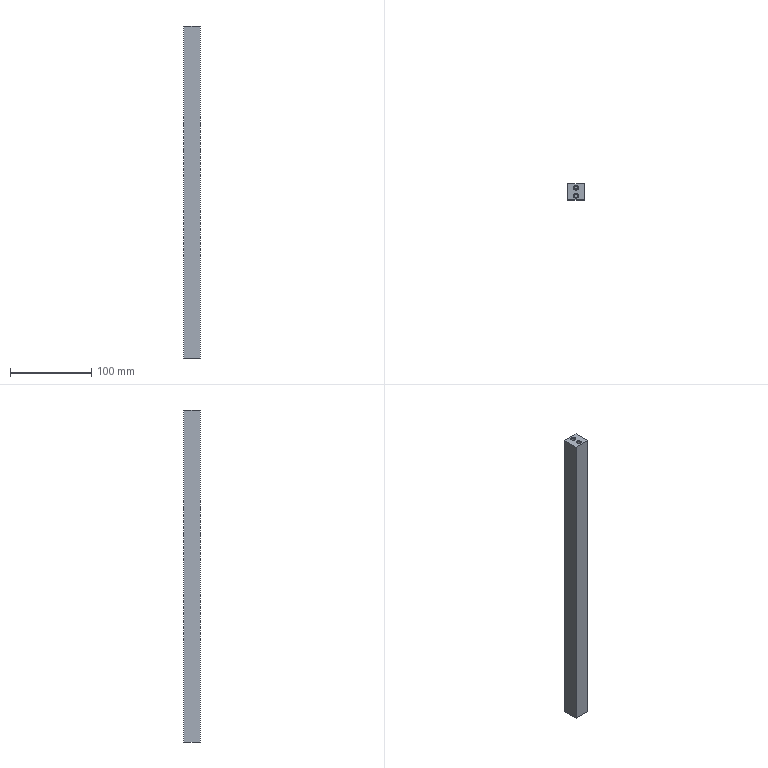Part | STEP file | Support rod | 1 solid | 26 faces | box 20 x 20 x 408 mm | volume 162668 mm3 | plane 10 | cone 8 | cylinder 8 | commonest cylinder face diameters 4 x8
STEP:
#1=CARTESIAN_POINT('',(-4.715,4.436,1.));
#2=VERTEX_POINT('',#1);
#3=CARTESIAN_POINT('',(-8.715,4.436,1.));
#4=VERTEX_POINT('',#3);
#5=CARTESIAN_POINT('',(-6.715,4.436,1.));
#6=DIRECTION('',(0.,0.,-1.));
#7=DIRECTION('',(-1.,0.,0.));
#8=AXIS2_PLACEMENT_3D('',#5,#6,#7);
#9=CIRCLE('',#8,2.);
#10=EDGE_CURVE('',#2,#4,#9,.T.);
#11=ORIENTED_EDGE('',*,*,#10,.F.);
#12=CARTESIAN_POINT('',(-3.715,4.436,0.));
#13=VERTEX_POINT('',#12);
#14=CARTESIAN_POINT('',(-3.715,4.436,0.));
#15=DIRECTION('',(0.7071,0.,-0.7071));
#16=VECTOR('',#15,1000.);
#17=LINE('',#14,#16);
#18=EDGE_CURVE('',#2,#13,#17,.T.);
#19=ORIENTED_EDGE('',*,*,#18,.T.);
#20=CARTESIAN_POINT('',(-9.715,4.436,0.));
#21=VERTEX_POINT('',#20);
#22=CARTESIAN_POINT('',(-6.715,4.436,0.));
#23=DIRECTION('',(0.,0.,-1.));
#24=DIRECTION('',(-1.,0.,0.));
#25=AXIS2_PLACEMENT_3D('',#22,#23,#24);
#26=CIRCLE('',#25,3.);
#27=EDGE_CURVE('',#13,#21,#26,.T.);
#28=ORIENTED_EDGE('',*,*,#27,.T.);
#29=CARTESIAN_POINT('',(-9.715,4.436,0.));
#30=DIRECTION('',(-0.7071,0.,-0.7071));
#31=VECTOR('',#30,1000.);
#32=LINE('',#29,#31);
#33=EDGE_CURVE('',#4,#21,#32,.T.);
#34=ORIENTED_EDGE('',*,*,#33,.F.);
#35=EDGE_LOOP('',(#11,#19,#28,#34));
#36=FACE_OUTER_BOUND('',#35,.T.);
#37=CARTESIAN_POINT('',(-6.715,4.436,0.));
#38=DIRECTION('',(0.,0.,-1.));
#39=DIRECTION('',(-1.,0.,0.));
#40=AXIS2_PLACEMENT_3D('',#37,#38,#39);
#41=CONICAL_SURFACE('',#40,3.,0.7854);
#42=ADVANCED_FACE('',(#36),#41,.F.);
#43=CARTESIAN_POINT('',(-4.715,-5.564,1.));
#44=VERTEX_POINT('',#43);
#45=CARTESIAN_POINT('',(-8.715,-5.564,1.));
#46=VERTEX_POINT('',#45);
#47=CARTESIAN_POINT('',(-6.715,-5.564,1.));
#48=DIRECTION('',(0.,0.,-1.));
#49=DIRECTION('',(-1.,0.,0.));
#50=AXIS2_PLACEMENT_3D('',#47,#48,#49);
#51=CIRCLE('',#50,2.);
#52=EDGE_CURVE('',#44,#46,#51,.T.);
#53=ORIENTED_EDGE('',*,*,#52,.F.);
#54=CARTESIAN_POINT('',(-3.715,-5.564,0.));
#55=VERTEX_POINT('',#54);
#56=CARTESIAN_POINT('',(-3.715,-5.564,0.));
#57=DIRECTION('',(0.7071,0.,-0.7071));
#58=VECTOR('',#57,1000.);
#59=LINE('',#56,#58);
#60=EDGE_CURVE('',#44,#55,#59,.T.);
#61=ORIENTED_EDGE('',*,*,#60,.T.);
#62=CARTESIAN_POINT('',(-9.715,-5.564,0.));
#63=VERTEX_POINT('',#62);
#64=CARTESIAN_POINT('',(-6.715,-5.564,0.));
#65=DIRECTION('',(0.,0.,-1.));
#66=DIRECTION('',(-1.,0.,0.));
#67=AXIS2_PLACEMENT_3D('',#64,#65,#66);
#68=CIRCLE('',#67,3.);
#69=EDGE_CURVE('',#55,#63,#68,.T.);
#70=ORIENTED_EDGE('',*,*,#69,.T.);
#71=CARTESIAN_POINT('',(-9.715,-5.564,0.));
#72=DIRECTION('',(-0.7071,0.,-0.7071));
#73=VECTOR('',#72,1000.);
#74=LINE('',#71,#73);
#75=EDGE_CURVE('',#46,#63,#74,.T.);
#76=ORIENTED_EDGE('',*,*,#75,.F.);
#77=EDGE_LOOP('',(#53,#61,#70,#76));
#78=FACE_OUTER_BOUND('',#77,.T.);
#79=CARTESIAN_POINT('',(-6.715,-5.564,0.));
#80=DIRECTION('',(0.,0.,-1.));
#81=DIRECTION('',(-1.,0.,0.));
#82=AXIS2_PLACEMENT_3D('',#79,#80,#81);
#83=CONICAL_SURFACE('',#82,3.,0.7854);
#84=ADVANCED_FACE('',(#78),#83,.F.);
#85=CARTESIAN_POINT('',(-6.715,6.436,407.));
#86=VERTEX_POINT('',#85);
#87=CARTESIAN_POINT('',(-8.715,4.436,407.));
#88=VERTEX_POINT('',#87);
#89=CARTESIAN_POINT('',(-6.715,4.436,407.));
#90=DIRECTION('',(0.,0.,1.));
#91=DIRECTION('',(1.,0.,0.));
#92=AXIS2_PLACEMENT_3D('',#89,#90,#91);
#93=CIRCLE('',#92,2.);
#94=EDGE_CURVE('',#86,#88,#93,.T.);
#95=ORIENTED_EDGE('',*,*,#94,.F.);
#96=CARTESIAN_POINT('',(-6.715,7.436,408.));
#97=VERTEX_POINT('',#96);
#98=CARTESIAN_POINT('',(-6.715,7.436,408.));
#99=DIRECTION('',(0.,0.7071,0.7071));
#100=VECTOR('',#99,1000.);
#101=LINE('',#98,#100);
#102=EDGE_CURVE('',#86,#97,#101,.T.);
#103=ORIENTED_EDGE('',*,*,#102,.T.);
#104=CARTESIAN_POINT('',(-6.715,1.436,408.));
#105=VERTEX_POINT('',#104);
#106=CARTESIAN_POINT('',(-6.715,4.436,408.));
#107=DIRECTION('',(0.,0.,-1.));
#108=DIRECTION('',(0.,-1.,0.));
#109=AXIS2_PLACEMENT_3D('',#106,#107,#108);
#110=CIRCLE('',#109,3.);
#111=EDGE_CURVE('',#105,#97,#110,.T.);
#112=ORIENTED_EDGE('',*,*,#111,.F.);
#113=CARTESIAN_POINT('',(-6.715,2.436,407.));
#114=VERTEX_POINT('',#113);
#115=CARTESIAN_POINT('',(-6.715,1.436,408.));
#116=DIRECTION('',(0.,-0.7071,0.7071));
#117=VECTOR('',#116,1000.);
#118=LINE('',#115,#117);
#119=EDGE_CURVE('',#114,#105,#118,.T.);
#120=ORIENTED_EDGE('',*,*,#119,.F.);
#121=CARTESIAN_POINT('',(-6.715,4.436,407.));
#122=DIRECTION('',(0.,0.,1.));
#123=DIRECTION('',(1.,0.,0.));
#124=AXIS2_PLACEMENT_3D('',#121,#122,#123);
#125=CIRCLE('',#124,2.);
#126=EDGE_CURVE('',#88,#114,#125,.T.);
#127=ORIENTED_EDGE('',*,*,#126,.F.);
#128=EDGE_LOOP('',(#95,#103,#112,#120,#127));
#129=FACE_OUTER_BOUND('',#128,.T.);
#130=CARTESIAN_POINT('',(-6.715,4.436,408.));
#131=DIRECTION('',(0.,0.,1.));
#132=DIRECTION('',(0.,-1.,0.));
#133=AXIS2_PLACEMENT_3D('',#130,#131,#132);
#134=CONICAL_SURFACE('',#133,3.,0.7854);
#135=ADVANCED_FACE('',(#129),#134,.F.);
#136=CARTESIAN_POINT('',(-6.715,-3.564,407.));
#137=VERTEX_POINT('',#136);
#138=CARTESIAN_POINT('',(-8.715,-5.564,407.));
#139=VERTEX_POINT('',#138);
#140=CARTESIAN_POINT('',(-6.715,-5.564,407.));
#141=DIRECTION('',(0.,0.,1.));
#142=DIRECTION('',(1.,0.,0.));
#143=AXIS2_PLACEMENT_3D('',#140,#141,#142);
#144=CIRCLE('',#143,2.);
#145=EDGE_CURVE('',#137,#139,#144,.T.);
#146=ORIENTED_EDGE('',*,*,#145,.F.);
#147=CARTESIAN_POINT('',(-6.715,-2.564,408.));
#148=VERTEX_POINT('',#147);
#149=CARTESIAN_POINT('',(-6.715,-2.564,408.));
#150=DIRECTION('',(0.,0.7071,0.7071));
#151=VECTOR('',#150,1000.);
#152=LINE('',#149,#151);
#153=EDGE_CURVE('',#137,#148,#152,.T.);
#154=ORIENTED_EDGE('',*,*,#153,.T.);
#155=CARTESIAN_POINT('',(-6.715,-8.564,408.));
#156=VERTEX_POINT('',#155);
#157=CARTESIAN_POINT('',(-6.715,-5.564,408.));
#158=DIRECTION('',(0.,0.,-1.));
#159=DIRECTION('',(0.,-1.,0.));
#160=AXIS2_PLACEMENT_3D('',#157,#158,#159);
#161=CIRCLE('',#160,3.);
#162=EDGE_CURVE('',#156,#148,#161,.T.);
#163=ORIENTED_EDGE('',*,*,#162,.F.);
#164=CARTESIAN_POINT('',(-6.715,-7.564,407.));
#165=VERTEX_POINT('',#164);
#166=CARTESIAN_POINT('',(-6.715,-8.564,408.));
#167=DIRECTION('',(0.,-0.7071,0.7071));
#168=VECTOR('',#167,1000.);
#169=LINE('',#166,#168);
#170=EDGE_CURVE('',#165,#156,#169,.T.);
#171=ORIENTED_EDGE('',*,*,#170,.F.);
#172=CARTESIAN_POINT('',(-6.715,-5.564,407.));
#173=DIRECTION('',(0.,0.,1.));
#174=DIRECTION('',(1.,0.,0.));
#175=AXIS2_PLACEMENT_3D('',#172,#173,#174);
#176=CIRCLE('',#175,2.);
#177=EDGE_CURVE('',#139,#165,#176,.T.);
#178=ORIENTED_EDGE('',*,*,#177,.F.);
#179=EDGE_LOOP('',(#146,#154,#163,#171,#178));
#180=FACE_OUTER_BOUND('',#179,.T.);
#181=CARTESIAN_POINT('',(-6.715,-5.564,408.));
#182=DIRECTION('',(0.,0.,1.));
#183=DIRECTION('',(0.,-1.,0.));
#184=AXIS2_PLACEMENT_3D('',#181,#182,#183);
#185=CONICAL_SURFACE('',#184,3.,0.7854);
#186=ADVANCED_FACE('',(#180),#185,.F.);
#187=CARTESIAN_POINT('',(-4.715,4.436,10.));
#188=VERTEX_POINT('',#187);
#189=CARTESIAN_POINT('',(-8.715,4.436,10.));
#190=VERTEX_POINT('',#189);
#191=CARTESIAN_POINT('',(-6.715,4.436,10.));
#192=DIRECTION('',(0.,0.,-1.));
#193=DIRECTION('',(-1.,0.,0.));
#194=AXIS2_PLACEMENT_3D('',#191,#192,#193);
#195=CIRCLE('',#194,2.);
#196=EDGE_CURVE('',#188,#190,#195,.T.);
#197=ORIENTED_EDGE('',*,*,#196,.F.);
#198=CARTESIAN_POINT('',(-4.715,4.436,10.));
#199=DIRECTION('',(0.,0.,-1.));
#200=VECTOR('',#199,1000.);
#201=LINE('',#198,#200);
#202=EDGE_CURVE('',#188,#2,#201,.T.);
#203=ORIENTED_EDGE('',*,*,#202,.T.);
#204=ORIENTED_EDGE('',*,*,#10,.T.);
#205=CARTESIAN_POINT('',(-8.715,4.436,10.));
#206=DIRECTION('',(0.,0.,-1.));
#207=VECTOR('',#206,1000.);
#208=LINE('',#205,#207);
#209=EDGE_CURVE('',#190,#4,#208,.T.);
#210=ORIENTED_EDGE('',*,*,#209,.F.);
#211=EDGE_LOOP('',(#197,#203,#204,#210));
#212=FACE_OUTER_BOUND('',#211,.T.);
#213=CARTESIAN_POINT('',(-6.715,4.436,10.));
#214=DIRECTION('',(0.,0.,-1.));
#215=DIRECTION('',(-1.,0.,0.));
#216=AXIS2_PLACEMENT_3D('',#213,#214,#215);
#217=CYLINDRICAL_SURFACE('',#216,2.);
#218=ADVANCED_FACE('',(#212),#217,.F.);
#219=CARTESIAN_POINT('',(-4.715,-5.564,10.));
#220=VERTEX_POINT('',#219);
#221=CARTESIAN_POINT('',(-8.715,-5.564,10.));
#222=VERTEX_POINT('',#221);
#223=CARTESIAN_POINT('',(-6.715,-5.564,10.));
#224=DIRECTION('',(0.,0.,-1.));
#225=DIRECTION('',(-1.,0.,0.));
#226=AXIS2_PLACEMENT_3D('',#223,#224,#225);
#227=CIRCLE('',#226,2.);
#228=EDGE_CURVE('',#220,#222,#227,.T.);
#229=ORIENTED_EDGE('',*,*,#228,.F.);
#230=CARTESIAN_POINT('',(-4.715,-5.564,10.));
#231=DIRECTION('',(0.,0.,-1.));
#232=VECTOR('',#231,1000.);
#233=LINE('',#230,#232);
#234=EDGE_CURVE('',#220,#44,#233,.T.);
#235=ORIENTED_EDGE('',*,*,#234,.T.);
#236=ORIENTED_EDGE('',*,*,#52,.T.);
#237=CARTESIAN_POINT('',(-8.715,-5.564,10.));
#238=DIRECTION('',(0.,0.,-1.));
#239=VECTOR('',#238,1000.);
#240=LINE('',#237,#239);
#241=EDGE_CURVE('',#222,#46,#240,.T.);
#242=ORIENTED_EDGE('',*,*,#241,.F.);
#243=EDGE_LOOP('',(#229,#235,#236,#242));
#244=FACE_OUTER_BOUND('',#243,.T.);
#245=CARTESIAN_POINT('',(-6.715,-5.564,10.));
#246=DIRECTION('',(0.,0.,-1.));
#247=DIRECTION('',(-1.,0.,0.));
#248=AXIS2_PLACEMENT_3D('',#245,#246,#247);
#249=CYLINDRICAL_SURFACE('',#248,2.);
#250=ADVANCED_FACE('',(#244),#249,.F.);
#251=CARTESIAN_POINT('',(-8.715,4.436,398.));
#252=VERTEX_POINT('',#251);
#253=CARTESIAN_POINT('',(-4.715,4.436,398.));
#254=VERTEX_POINT('',#253);
#255=CARTESIAN_POINT('',(-6.715,4.436,398.));
#256=DIRECTION('',(0.,0.,1.));
#257=DIRECTION('',(1.,0.,0.));
#258=AXIS2_PLACEMENT_3D('',#255,#256,#257);
#259=CIRCLE('',#258,2.);
#260=EDGE_CURVE('',#252,#254,#259,.T.);
#261=ORIENTED_EDGE('',*,*,#260,.F.);
#262=CARTESIAN_POINT('',(-8.715,4.436,398.));
#263=DIRECTION('',(0.,0.,1.));
#264=VECTOR('',#263,1000.);
#265=LINE('',#262,#264);
#266=EDGE_CURVE('',#252,#88,#265,.T.);
#267=ORIENTED_EDGE('',*,*,#266,.T.);
#268=ORIENTED_EDGE('',*,*,#126,.T.);
#269=CARTESIAN_POINT('',(-4.715,4.436,407.));
#270=VERTEX_POINT('',#269);
#271=CARTESIAN_POINT('',(-6.715,4.436,407.));
#272=DIRECTION('',(0.,0.,1.));
#273=DIRECTION('',(1.,0.,0.));
#274=AXIS2_PLACEMENT_3D('',#271,#272,#273);
#275=CIRCLE('',#274,2.);
#276=EDGE_CURVE('',#114,#270,#275,.T.);
#277=ORIENTED_EDGE('',*,*,#276,.T.);
#278=CARTESIAN_POINT('',(-4.715,4.436,398.));
#279=DIRECTION('',(0.,0.,1.));
#280=VECTOR('',#279,1000.);
#281=LINE('',#278,#280);
#282=EDGE_CURVE('',#254,#270,#281,.T.);
#283=ORIENTED_EDGE('',*,*,#282,.F.);
#284=EDGE_LOOP('',(#261,#267,#268,#277,#283));
#285=FACE_OUTER_BOUND('',#284,.T.);
#286=CARTESIAN_POINT('',(-6.715,4.436,398.));
#287=DIRECTION('',(0.,0.,1.));
#288=DIRECTION('',(1.,0.,0.));
#289=AXIS2_PLACEMENT_3D('',#286,#287,#288);
#290=CYLINDRICAL_SURFACE('',#289,2.);
#291=ADVANCED_FACE('',(#285),#290,.F.);
#292=CARTESIAN_POINT('',(-8.715,-5.564,398.));
#293=VERTEX_POINT('',#292);
#294=CARTESIAN_POINT('',(-4.715,-5.564,398.));
#295=VERTEX_POINT('',#294);
#296=CARTESIAN_POINT('',(-6.715,-5.564,398.));
#297=DIRECTION('',(0.,0.,1.));
#298=DIRECTION('',(1.,0.,0.));
#299=AXIS2_PLACEMENT_3D('',#296,#297,#298);
#300=CIRCLE('',#299,2.);
#301=EDGE_CURVE('',#293,#295,#300,.T.);
#302=ORIENTED_EDGE('',*,*,#301,.F.);
#303=CARTESIAN_POINT('',(-8.715,-5.564,398.));
#304=DIRECTION('',(0.,0.,1.));
#305=VECTOR('',#304,1000.);
#306=LINE('',#303,#305);
#307=EDGE_CURVE('',#293,#139,#306,.T.);
#308=ORIENTED_EDGE('',*,*,#307,.T.);
#309=ORIENTED_EDGE('',*,*,#177,.T.);
#310=CARTESIAN_POINT('',(-4.715,-5.564,407.));
#311=VERTEX_POINT('',#310);
#312=CARTESIAN_POINT('',(-6.715,-5.564,407.));
#313=DIRECTION('',(0.,0.,1.));
#314=DIRECTION('',(1.,0.,0.));
#315=AXIS2_PLACEMENT_3D('',#312,#313,#314);
#316=CIRCLE('',#315,2.);
#317=EDGE_CURVE('',#165,#311,#316,.T.);
#318=ORIENTED_EDGE('',*,*,#317,.T.);
#319=CARTESIAN_POINT('',(-4.715,-5.564,398.));
#320=DIRECTION('',(0.,0.,1.));
#321=VECTOR('',#320,1000.);
#322=LINE('',#319,#321);
#323=EDGE_CURVE('',#295,#311,#322,.T.);
#324=ORIENTED_EDGE('',*,*,#323,.F.);
#325=EDGE_LOOP('',(#302,#308,#309,#318,#324));
#326=FACE_OUTER_BOUND('',#325,.T.);
#327=CARTESIAN_POINT('',(-6.715,-5.564,398.));
#328=DIRECTION('',(0.,0.,1.));
#329=DIRECTION('',(1.,0.,0.));
#330=AXIS2_PLACEMENT_3D('',#327,#328,#329);
#331=CYLINDRICAL_SURFACE('',#330,2.);
#332=ADVANCED_FACE('',(#326),#331,.F.);
#333=CARTESIAN_POINT('',(-16.715,-10.564,408.));
#334=VERTEX_POINT('',#333);
#335=CARTESIAN_POINT('',(-16.715,-10.564,0.));
#336=VERTEX_POINT('',#335);
#337=CARTESIAN_POINT('',(-16.715,-10.564,408.));
#338=DIRECTION('',(0.,0.,-1.));
#339=VECTOR('',#338,1000.);
#340=LINE('',#337,#339);
#341=EDGE_CURVE('',#334,#336,#340,.T.);
#342=ORIENTED_EDGE('',*,*,#341,.F.);
#343=CARTESIAN_POINT('',(-16.715,9.436,408.));
#344=VERTEX_POINT('',#343);
#345=CARTESIAN_POINT('',(-16.715,9.436,408.));
#346=DIRECTION('',(0.,-1.,0.));
#347=VECTOR('',#346,1000.);
#348=LINE('',#345,#347);
#349=EDGE_CURVE('',#344,#334,#348,.T.);
#350=ORIENTED_EDGE('',*,*,#349,.F.);
#351=CARTESIAN_POINT('',(-16.715,9.436,0.));
#352=VERTEX_POINT('',#351);
#353=CARTESIAN_POINT('',(-16.715,9.436,408.));
#354=DIRECTION('',(0.,0.,1.));
#355=VECTOR('',#354,1000.);
#356=LINE('',#353,#355);
#357=EDGE_CURVE('',#352,#344,#356,.T.);
#358=ORIENTED_EDGE('',*,*,#357,.F.);
#359=CARTESIAN_POINT('',(-16.715,9.436,0.));
#360=DIRECTION('',(0.,1.,0.));
#361=VECTOR('',#360,1000.);
#362=LINE('',#359,#361);
#363=EDGE_CURVE('',#336,#352,#362,.T.);
#364=ORIENTED_EDGE('',*,*,#363,.F.);
#365=EDGE_LOOP('',(#342,#350,#358,#364));
#366=FACE_OUTER_BOUND('',#365,.T.);
#367=CARTESIAN_POINT('',(-16.715,9.436,408.));
#368=DIRECTION('',(1.,0.,0.));
#369=DIRECTION('',(0.,0.,-1.));
#370=AXIS2_PLACEMENT_3D('',#367,#368,#369);
#371=PLANE('',#370);
#372=ADVANCED_FACE('',(#366),#371,.F.);
#373=CARTESIAN_POINT('',(3.285,9.436,0.));
#374=VERTEX_POINT('',#373);
#375=CARTESIAN_POINT('',(-16.715,9.436,0.));
#376=DIRECTION('',(-1.,0.,0.));
#377=VECTOR('',#376,1000.);
#378=LINE('',#375,#377);
#379=EDGE_CURVE('',#374,#352,#378,.T.);
#380=ORIENTED_EDGE('',*,*,#379,.F.);
#381=CARTESIAN_POINT('',(3.285,-10.564,0.));
#382=VERTEX_POINT('',#381);
#383=CARTESIAN_POINT('',(3.285,-10.564,0.));
#384=DIRECTION('',(0.,1.,0.));
#385=VECTOR('',#384,1000.);
#386=LINE('',#383,#385);
#387=EDGE_CURVE('',#382,#374,#386,.T.);
#388=ORIENTED_EDGE('',*,*,#387,.F.);
#389=CARTESIAN_POINT('',(-16.715,-10.564,0.));
#390=DIRECTION('',(1.,0.,0.));
#391=VECTOR('',#390,1000.);
#392=LINE('',#389,#391);
#393=EDGE_CURVE('',#336,#382,#392,.T.);
#394=ORIENTED_EDGE('',*,*,#393,.F.);
#395=ORIENTED_EDGE('',*,*,#363,.T.);
#396=EDGE_LOOP('',(#380,#388,#394,#395));
#397=FACE_OUTER_BOUND('',#396,.T.);
#398=CARTESIAN_POINT('',(-6.715,4.436,0.));
#399=DIRECTION('',(0.,0.,-1.));
#400=DIRECTION('',(-1.,0.,0.));
#401=AXIS2_PLACEMENT_3D('',#398,#399,#400);
#402=CIRCLE('',#401,3.);
#403=EDGE_CURVE('',#21,#13,#402,.T.);
#404=ORIENTED_EDGE('',*,*,#403,.F.);
#405=ORIENTED_EDGE('',*,*,#27,.F.);
#406=EDGE_LOOP('',(#404,#405));
#407=FACE_BOUND('',#406,.T.);
#408=CARTESIAN_POINT('',(-6.715,-5.564,0.));
#409=DIRECTION('',(0.,0.,-1.));
#410=DIRECTION('',(-1.,0.,0.));
#411=AXIS2_PLACEMENT_3D('',#408,#409,#410);
#412=CIRCLE('',#411,3.);
#413=EDGE_CURVE('',#63,#55,#412,.T.);
#414=ORIENTED_EDGE('',*,*,#413,.F.);
#415=ORIENTED_EDGE('',*,*,#69,.F.);
#416=EDGE_LOOP('',(#414,#415));
#417=FACE_BOUND('',#416,.T.);
#418=CARTESIAN_POINT('',(-16.715,-10.564,0.));
#419=DIRECTION('',(0.,0.,1.));
#420=DIRECTION('',(1.,0.,0.));
#421=AXIS2_PLACEMENT_3D('',#418,#419,#420);
#422=PLANE('',#421);
#423=ADVANCED_FACE('',(#397,#407,#417),#422,.F.);
#424=CARTESIAN_POINT('',(3.285,-10.564,408.));
#425=VERTEX_POINT('',#424);
#426=CARTESIAN_POINT('',(3.285,-10.564,408.));
#427=DIRECTION('',(0.,0.,-1.));
#428=VECTOR('',#427,1000.);
#429=LINE('',#426,#428);
#430=EDGE_CURVE('',#425,#382,#429,.T.);
#431=ORIENTED_EDGE('',*,*,#430,.F.);
#432=CARTESIAN_POINT('',(-16.715,-10.564,408.));
#433=DIRECTION('',(1.,0.,0.));
#434=VECTOR('',#433,1000.);
#435=LINE('',#432,#434);
#436=EDGE_CURVE('',#334,#425,#435,.T.);
#437=ORIENTED_EDGE('',*,*,#436,.F.);
#438=ORIENTED_EDGE('',*,*,#341,.T.);
#439=ORIENTED_EDGE('',*,*,#393,.T.);
#440=EDGE_LOOP('',(#431,#437,#438,#439));
#441=FACE_OUTER_BOUND('',#440,.T.);
#442=CARTESIAN_POINT('',(-16.715,-10.564,408.));
#443=DIRECTION('',(0.,1.,0.));
#444=DIRECTION('',(0.,0.,1.));
#445=AXIS2_PLACEMENT_3D('',#442,#443,#444);
#446=PLANE('',#445);
#447=ADVANCED_FACE('',(#441),#446,.F.);
#448=CARTESIAN_POINT('',(3.285,9.436,408.));
#449=VERTEX_POINT('',#448);
#450=CARTESIAN_POINT('',(3.285,-10.564,408.));
#451=DIRECTION('',(0.,1.,0.));
#452=VECTOR('',#451,1000.);
#453=LINE('',#450,#452);
#454=EDGE_CURVE('',#425,#449,#453,.T.);
#455=ORIENTED_EDGE('',*,*,#454,.T.);
#456=CARTESIAN_POINT('',(-16.715,9.436,408.));
#457=DIRECTION('',(-1.,0.,0.));
#458=VECTOR('',#457,1000.);
#459=LINE('',#456,#458);
#460=EDGE_CURVE('',#449,#344,#459,.T.);
#461=ORIENTED_EDGE('',*,*,#460,.T.);
#462=ORIENTED_EDGE('',*,*,#349,.T.);
#463=ORIENTED_EDGE('',*,*,#436,.T.);
#464=EDGE_LOOP('',(#455,#461,#462,#463));
#465=FACE_OUTER_BOUND('',#464,.T.);
#466=ORIENTED_EDGE('',*,*,#111,.T.);
#467=CARTESIAN_POINT('',(-6.715,4.436,408.));
#468=DIRECTION('',(0.,0.,-1.));
#469=DIRECTION('',(0.,-1.,0.));
#470=AXIS2_PLACEMENT_3D('',#467,#468,#469);
#471=CIRCLE('',#470,3.);
#472=EDGE_CURVE('',#97,#105,#471,.T.);
#473=ORIENTED_EDGE('',*,*,#472,.T.);
#474=EDGE_LOOP('',(#466,#473));
#475=FACE_BOUND('',#474,.T.);
#476=ORIENTED_EDGE('',*,*,#162,.T.);
#477=CARTESIAN_POINT('',(-6.715,-5.564,408.));
#478=DIRECTION('',(0.,0.,-1.));
#479=DIRECTION('',(0.,-1.,0.));
#480=AXIS2_PLACEMENT_3D('',#477,#478,#479);
#481=CIRCLE('',#480,3.);
#482=EDGE_CURVE('',#148,#156,#481,.T.);
#483=ORIENTED_EDGE('',*,*,#482,.T.);
#484=EDGE_LOOP('',(#476,#483));
#485=FACE_BOUND('',#484,.T.);
#486=CARTESIAN_POINT('',(-16.715,-10.564,408.));
#487=DIRECTION('',(0.,0.,1.));
#488=DIRECTION('',(1.,0.,0.));
#489=AXIS2_PLACEMENT_3D('',#486,#487,#488);
#490=PLANE('',#489);
#491=ADVANCED_FACE('',(#465,#475,#485),#490,.T.);
#492=ORIENTED_EDGE('',*,*,#357,.T.);
#493=ORIENTED_EDGE('',*,*,#460,.F.);
#494=CARTESIAN_POINT('',(3.285,9.436,408.));
#495=DIRECTION('',(0.,0.,1.));
#496=VECTOR('',#495,1000.);
#497=LINE('',#494,#496);
#498=EDGE_CURVE('',#374,#449,#497,.T.);
#499=ORIENTED_EDGE('',*,*,#498,.F.);
#500=ORIENTED_EDGE('',*,*,#379,.T.);
#501=EDGE_LOOP('',(#492,#493,#499,#500));
#502=FACE_OUTER_BOUND('',#501,.T.);
#503=CARTESIAN_POINT('',(-16.715,9.436,408.));
#504=DIRECTION('',(0.,-1.,0.));
#505=DIRECTION('',(0.,0.,-1.));
#506=AXIS2_PLACEMENT_3D('',#503,#504,#505);
#507=PLANE('',#506);
#508=ADVANCED_FACE('',(#502),#507,.F.);
#509=ORIENTED_EDGE('',*,*,#498,.T.);
#510=ORIENTED_EDGE('',*,*,#454,.F.);
#511=ORIENTED_EDGE('',*,*,#430,.T.);
#512=ORIENTED_EDGE('',*,*,#387,.T.);
#513=EDGE_LOOP('',(#509,#510,#511,#512));
#514=FACE_OUTER_BOUND('',#513,.T.);
#515=CARTESIAN_POINT('',(3.285,9.436,408.));
#516=DIRECTION('',(-1.,0.,0.));
#517=DIRECTION('',(0.,0.,1.));
#518=AXIS2_PLACEMENT_3D('',#515,#516,#517);
#519=PLANE('',#518);
#520=ADVANCED_FACE('',(#514),#519,.F.);
#521=ORIENTED_EDGE('',*,*,#18,.F.);
#522=CARTESIAN_POINT('',(-6.715,4.436,1.));
#523=DIRECTION('',(0.,0.,-1.));
#524=DIRECTION('',(-1.,0.,0.));
#525=AXIS2_PLACEMENT_3D('',#522,#523,#524);
#526=CIRCLE('',#525,2.);
#527=EDGE_CURVE('',#4,#2,#526,.T.);
#528=ORIENTED_EDGE('',*,*,#527,.F.);
#529=ORIENTED_EDGE('',*,*,#33,.T.);
#530=ORIENTED_EDGE('',*,*,#403,.T.);
#531=EDGE_LOOP('',(#521,#528,#529,#530));
#532=FACE_OUTER_BOUND('',#531,.T.);
#533=CARTESIAN_POINT('',(-6.715,4.436,0.));
#534=DIRECTION('',(0.,0.,-1.));
#535=DIRECTION('',(-1.,0.,0.));
#536=AXIS2_PLACEMENT_3D('',#533,#534,#535);
#537=CONICAL_SURFACE('',#536,3.,0.7854);
#538=ADVANCED_FACE('',(#532),#537,.F.);
#539=ORIENTED_EDGE('',*,*,#60,.F.);
#540=CARTESIAN_POINT('',(-6.715,-5.564,1.));
#541=DIRECTION('',(0.,0.,-1.));
#542=DIRECTION('',(-1.,0.,0.));
#543=AXIS2_PLACEMENT_3D('',#540,#541,#542);
#544=CIRCLE('',#543,2.);
#545=EDGE_CURVE('',#46,#44,#544,.T.);
#546=ORIENTED_EDGE('',*,*,#545,.F.);
#547=ORIENTED_EDGE('',*,*,#75,.T.);
#548=ORIENTED_EDGE('',*,*,#413,.T.);
#549=EDGE_LOOP('',(#539,#546,#547,#548));
#550=FACE_OUTER_BOUND('',#549,.T.);
#551=CARTESIAN_POINT('',(-6.715,-5.564,0.));
#552=DIRECTION('',(0.,0.,-1.));
#553=DIRECTION('',(-1.,0.,0.));
#554=AXIS2_PLACEMENT_3D('',#551,#552,#553);
#555=CONICAL_SURFACE('',#554,3.,0.7854);
#556=ADVANCED_FACE('',(#550),#555,.F.);
#557=ORIENTED_EDGE('',*,*,#102,.F.);
#558=CARTESIAN_POINT('',(-6.715,4.436,407.));
#559=DIRECTION('',(0.,0.,1.));
#560=DIRECTION('',(1.,0.,0.));
#561=AXIS2_PLACEMENT_3D('',#558,#559,#560);
#562=CIRCLE('',#561,2.);
#563=EDGE_CURVE('',#270,#86,#562,.T.);
#564=ORIENTED_EDGE('',*,*,#563,.F.);
#565=ORIENTED_EDGE('',*,*,#276,.F.);
#566=ORIENTED_EDGE('',*,*,#119,.T.);
#567=ORIENTED_EDGE('',*,*,#472,.F.);
#568=EDGE_LOOP('',(#557,#564,#565,#566,#567));
#569=FACE_OUTER_BOUND('',#568,.T.);
#570=CARTESIAN_POINT('',(-6.715,4.436,408.));
#571=DIRECTION('',(0.,0.,1.));
#572=DIRECTION('',(0.,-1.,0.));
#573=AXIS2_PLACEMENT_3D('',#570,#571,#572);
#574=CONICAL_SURFACE('',#573,3.,0.7854);
#575=ADVANCED_FACE('',(#569),#574,.F.);
#576=ORIENTED_EDGE('',*,*,#153,.F.);
#577=CARTESIAN_POINT('',(-6.715,-5.564,407.));
#578=DIRECTION('',(0.,0.,1.));
#579=DIRECTION('',(1.,0.,0.));
#580=AXIS2_PLACEMENT_3D('',#577,#578,#579);
#581=CIRCLE('',#580,2.);
#582=EDGE_CURVE('',#311,#137,#581,.T.);
#583=ORIENTED_EDGE('',*,*,#582,.F.);
#584=ORIENTED_EDGE('',*,*,#317,.F.);
#585=ORIENTED_EDGE('',*,*,#170,.T.);
#586=ORIENTED_EDGE('',*,*,#482,.F.);
#587=EDGE_LOOP('',(#576,#583,#584,#585,#586));
#588=FACE_OUTER_BOUND('',#587,.T.);
#589=CARTESIAN_POINT('',(-6.715,-5.564,408.));
#590=DIRECTION('',(0.,0.,1.));
#591=DIRECTION('',(0.,-1.,0.));
#592=AXIS2_PLACEMENT_3D('',#589,#590,#591);
#593=CONICAL_SURFACE('',#592,3.,0.7854);
#594=ADVANCED_FACE('',(#588),#593,.F.);
#595=ORIENTED_EDGE('',*,*,#202,.F.);
#596=CARTESIAN_POINT('',(-6.715,4.436,10.));
#597=DIRECTION('',(0.,0.,-1.));
#598=DIRECTION('',(-1.,0.,0.));
#599=AXIS2_PLACEMENT_3D('',#596,#597,#598);
#600=CIRCLE('',#599,2.);
#601=EDGE_CURVE('',#190,#188,#600,.T.);
#602=ORIENTED_EDGE('',*,*,#601,.F.);
#603=ORIENTED_EDGE('',*,*,#209,.T.);
#604=ORIENTED_EDGE('',*,*,#527,.T.);
#605=EDGE_LOOP('',(#595,#602,#603,#604));
#606=FACE_OUTER_BOUND('',#605,.T.);
#607=CARTESIAN_POINT('',(-6.715,4.436,10.));
#608=DIRECTION('',(0.,0.,-1.));
#609=DIRECTION('',(-1.,0.,0.));
#610=AXIS2_PLACEMENT_3D('',#607,#608,#609);
#611=CYLINDRICAL_SURFACE('',#610,2.);
#612=ADVANCED_FACE('',(#606),#611,.F.);
#613=ORIENTED_EDGE('',*,*,#234,.F.);
#614=CARTESIAN_POINT('',(-6.715,-5.564,10.));
#615=DIRECTION('',(0.,0.,-1.));
#616=DIRECTION('',(-1.,0.,0.));
#617=AXIS2_PLACEMENT_3D('',#614,#615,#616);
#618=CIRCLE('',#617,2.);
#619=EDGE_CURVE('',#222,#220,#618,.T.);
#620=ORIENTED_EDGE('',*,*,#619,.F.);
#621=ORIENTED_EDGE('',*,*,#241,.T.);
#622=ORIENTED_EDGE('',*,*,#545,.T.);
#623=EDGE_LOOP('',(#613,#620,#621,#622));
#624=FACE_OUTER_BOUND('',#623,.T.);
#625=CARTESIAN_POINT('',(-6.715,-5.564,10.));
#626=DIRECTION('',(0.,0.,-1.));
#627=DIRECTION('',(-1.,0.,0.));
#628=AXIS2_PLACEMENT_3D('',#625,#626,#627);
#629=CYLINDRICAL_SURFACE('',#628,2.);
#630=ADVANCED_FACE('',(#624),#629,.F.);
#631=ORIENTED_EDGE('',*,*,#266,.F.);
#632=CARTESIAN_POINT('',(-6.715,4.436,398.));
#633=DIRECTION('',(0.,0.,1.));
#634=DIRECTION('',(1.,0.,0.));
#635=AXIS2_PLACEMENT_3D('',#632,#633,#634);
#636=CIRCLE('',#635,2.);
#637=EDGE_CURVE('',#254,#252,#636,.T.);
#638=ORIENTED_EDGE('',*,*,#637,.F.);
#639=ORIENTED_EDGE('',*,*,#282,.T.);
#640=ORIENTED_EDGE('',*,*,#563,.T.);
#641=ORIENTED_EDGE('',*,*,#94,.T.);
#642=EDGE_LOOP('',(#631,#638,#639,#640,#641));
#643=FACE_OUTER_BOUND('',#642,.T.);
#644=CARTESIAN_POINT('',(-6.715,4.436,398.));
#645=DIRECTION('',(0.,0.,1.));
#646=DIRECTION('',(1.,0.,0.));
#647=AXIS2_PLACEMENT_3D('',#644,#645,#646);
#648=CYLINDRICAL_SURFACE('',#647,2.);
#649=ADVANCED_FACE('',(#643),#648,.F.);
#650=ORIENTED_EDGE('',*,*,#307,.F.);
#651=CARTESIAN_POINT('',(-6.715,-5.564,398.));
#652=DIRECTION('',(0.,0.,1.));
#653=DIRECTION('',(1.,0.,0.));
#654=AXIS2_PLACEMENT_3D('',#651,#652,#653);
#655=CIRCLE('',#654,2.);
#656=EDGE_CURVE('',#295,#293,#655,.T.);
#657=ORIENTED_EDGE('',*,*,#656,.F.);
#658=ORIENTED_EDGE('',*,*,#323,.T.);
#659=ORIENTED_EDGE('',*,*,#582,.T.);
#660=ORIENTED_EDGE('',*,*,#145,.T.);
#661=EDGE_LOOP('',(#650,#657,#658,#659,#660));
#662=FACE_OUTER_BOUND('',#661,.T.);
#663=CARTESIAN_POINT('',(-6.715,-5.564,398.));
#664=DIRECTION('',(0.,0.,1.));
#665=DIRECTION('',(1.,0.,0.));
#666=AXIS2_PLACEMENT_3D('',#663,#664,#665);
#667=CYLINDRICAL_SURFACE('',#666,2.);
#668=ADVANCED_FACE('',(#662),#667,.F.);
#669=ORIENTED_EDGE('',*,*,#601,.T.);
#670=ORIENTED_EDGE('',*,*,#196,.T.);
#671=EDGE_LOOP('',(#669,#670));
#672=FACE_OUTER_BOUND('',#671,.T.);
#673=CARTESIAN_POINT('',(-6.715,4.436,10.));
#674=DIRECTION('',(0.,0.,-1.));
#675=DIRECTION('',(-1.,0.,0.));
#676=AXIS2_PLACEMENT_3D('',#673,#674,#675);
#677=PLANE('',#676);
#678=ADVANCED_FACE('',(#672),#677,.T.);
#679=ORIENTED_EDGE('',*,*,#619,.T.);
#680=ORIENTED_EDGE('',*,*,#228,.T.);
#681=EDGE_LOOP('',(#679,#680));
#682=FACE_OUTER_BOUND('',#681,.T.);
#683=CARTESIAN_POINT('',(-6.715,-5.564,10.));
#684=DIRECTION('',(0.,0.,-1.));
#685=DIRECTION('',(-1.,0.,0.));
#686=AXIS2_PLACEMENT_3D('',#683,#684,#685);
#687=PLANE('',#686);
#688=ADVANCED_FACE('',(#682),#687,.T.);
#689=ORIENTED_EDGE('',*,*,#637,.T.);
#690=ORIENTED_EDGE('',*,*,#260,.T.);
#691=EDGE_LOOP('',(#689,#690));
#692=FACE_OUTER_BOUND('',#691,.T.);
#693=CARTESIAN_POINT('',(-6.715,4.436,398.));
#694=DIRECTION('',(0.,0.,1.));
#695=DIRECTION('',(1.,0.,0.));
#696=AXIS2_PLACEMENT_3D('',#693,#694,#695);
#697=PLANE('',#696);
#698=ADVANCED_FACE('',(#692),#697,.T.);
#699=ORIENTED_EDGE('',*,*,#656,.T.);
#700=ORIENTED_EDGE('',*,*,#301,.T.);
#701=EDGE_LOOP('',(#699,#700));
#702=FACE_OUTER_BOUND('',#701,.T.);
#703=CARTESIAN_POINT('',(-6.715,-5.564,398.));
#704=DIRECTION('',(0.,0.,1.));
#705=DIRECTION('',(1.,0.,0.));
#706=AXIS2_PLACEMENT_3D('',#703,#704,#705);
#707=PLANE('',#706);
#708=ADVANCED_FACE('',(#702),#707,.T.);
#709=CLOSED_SHELL('',(#42,#84,#135,#186,#218,#250,#291,#332,#372,#423,#447,#491,#508,#520,#538,#556,#575,#594,#612,#630,#649,#668,#678,#688,#698,#708));
#710=MANIFOLD_SOLID_BREP('',#709);
#711=CARTESIAN_POINT('',(0.,0.,0.));
#712=DIRECTION('',(0.,0.,1.));
#713=DIRECTION('',(1.,0.,0.));
#714=AXIS2_PLACEMENT_3D('',#711,#712,#713);
#715=(LENGTH_UNIT()NAMED_UNIT(*)SI_UNIT(.MILLI.,.METRE.));
#716=UNCERTAINTY_MEASURE_WITH_UNIT(LENGTH_MEASURE(0.00001),#715,'','');
#717=(NAMED_UNIT(*)PLANE_ANGLE_UNIT()SI_UNIT($,.RADIAN.));
#718=(NAMED_UNIT(*)SI_UNIT($,.STERADIAN.)SOLID_ANGLE_UNIT());
#719=(GEOMETRIC_REPRESENTATION_CONTEXT(3)GLOBAL_UNCERTAINTY_ASSIGNED_CONTEXT((#716))GLOBAL_UNIT_ASSIGNED_CONTEXT((#715,#717,#718))REPRESENTATION_CONTEXT('',''));
#720=ADVANCED_BREP_SHAPE_REPRESENTATION('',(#710,#714),#719);